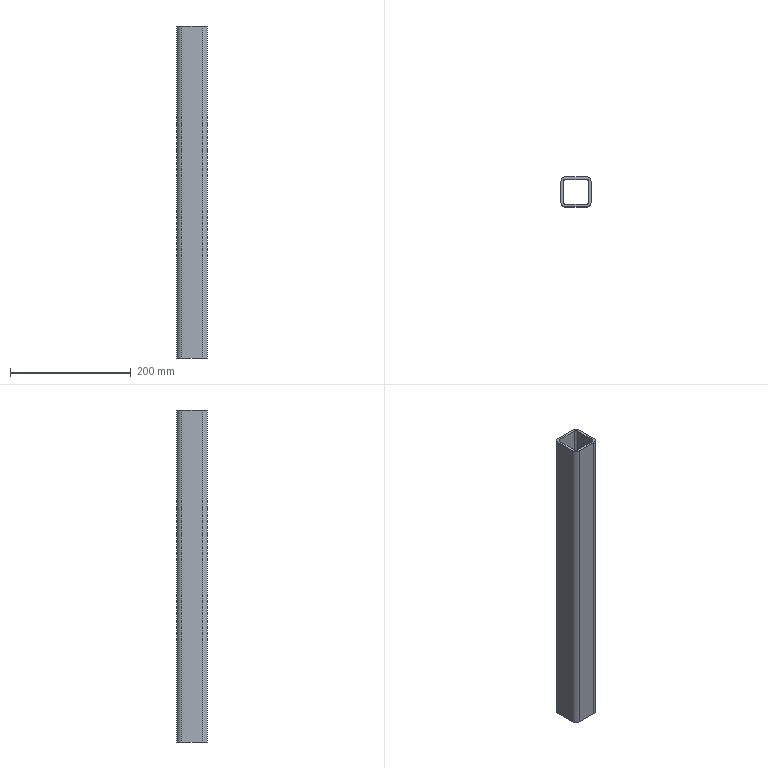Part | SolidWorks | features Extrusion 1 | 1 solid | 18 faces | box 50 x 50 x 550 mm | volume 382138 mm3 | plane 10 | cylinder 8 | commonest cylinder face diameters 8 x4 16 x4
STEP:
#1=CARTESIAN_POINT('',(17.,-25.,275.));
#2=VERTEX_POINT('',#1);
#3=CARTESIAN_POINT('',(25.,-17.,275.));
#4=VERTEX_POINT('',#3);
#5=CARTESIAN_POINT('',(17.,-17.,275.));
#6=DIRECTION('',(0.,0.,1.));
#7=DIRECTION('',(1.,0.,0.));
#8=AXIS2_PLACEMENT_3D('',#5,#6,#7);
#9=CIRCLE('',#8,8.);
#10=EDGE_CURVE('',#2,#4,#9,.T.);
#11=ORIENTED_EDGE('',*,*,#10,.T.);
#12=CARTESIAN_POINT('',(25.,17.,275.));
#13=VERTEX_POINT('',#12);
#14=CARTESIAN_POINT('',(25.,-17.,275.));
#15=DIRECTION('',(0.,1.,0.));
#16=VECTOR('',#15,1000.);
#17=LINE('',#14,#16);
#18=EDGE_CURVE('',#4,#13,#17,.T.);
#19=ORIENTED_EDGE('',*,*,#18,.T.);
#20=CARTESIAN_POINT('',(17.,25.,275.));
#21=VERTEX_POINT('',#20);
#22=CARTESIAN_POINT('',(17.,17.,275.));
#23=DIRECTION('',(0.,0.,1.));
#24=DIRECTION('',(-1.,0.,0.));
#25=AXIS2_PLACEMENT_3D('',#22,#23,#24);
#26=CIRCLE('',#25,8.);
#27=EDGE_CURVE('',#13,#21,#26,.T.);
#28=ORIENTED_EDGE('',*,*,#27,.T.);
#29=CARTESIAN_POINT('',(-17.,25.,275.));
#30=VERTEX_POINT('',#29);
#31=CARTESIAN_POINT('',(-17.,25.,275.));
#32=DIRECTION('',(-1.,0.,0.));
#33=VECTOR('',#32,1000.);
#34=LINE('',#31,#33);
#35=EDGE_CURVE('',#21,#30,#34,.T.);
#36=ORIENTED_EDGE('',*,*,#35,.T.);
#37=CARTESIAN_POINT('',(-25.,17.,275.));
#38=VERTEX_POINT('',#37);
#39=CARTESIAN_POINT('',(-17.,17.,275.));
#40=DIRECTION('',(0.,0.,1.));
#41=DIRECTION('',(-1.,0.,0.));
#42=AXIS2_PLACEMENT_3D('',#39,#40,#41);
#43=CIRCLE('',#42,8.);
#44=EDGE_CURVE('',#30,#38,#43,.T.);
#45=ORIENTED_EDGE('',*,*,#44,.T.);
#46=CARTESIAN_POINT('',(-25.,-17.,275.));
#47=VERTEX_POINT('',#46);
#48=CARTESIAN_POINT('',(-25.,-17.,275.));
#49=DIRECTION('',(0.,-1.,0.));
#50=VECTOR('',#49,1000.);
#51=LINE('',#48,#50);
#52=EDGE_CURVE('',#38,#47,#51,.T.);
#53=ORIENTED_EDGE('',*,*,#52,.T.);
#54=CARTESIAN_POINT('',(-17.,-25.,275.));
#55=VERTEX_POINT('',#54);
#56=CARTESIAN_POINT('',(-17.,-17.,275.));
#57=DIRECTION('',(0.,0.,1.));
#58=DIRECTION('',(-1.,0.,0.));
#59=AXIS2_PLACEMENT_3D('',#56,#57,#58);
#60=CIRCLE('',#59,8.);
#61=EDGE_CURVE('',#47,#55,#60,.T.);
#62=ORIENTED_EDGE('',*,*,#61,.T.);
#63=CARTESIAN_POINT('',(-17.,-25.,275.));
#64=DIRECTION('',(1.,0.,0.));
#65=VECTOR('',#64,1000.);
#66=LINE('',#63,#65);
#67=EDGE_CURVE('',#55,#2,#66,.T.);
#68=ORIENTED_EDGE('',*,*,#67,.T.);
#69=EDGE_LOOP('',(#11,#19,#28,#36,#45,#53,#62,#68));
#70=FACE_OUTER_BOUND('',#69,.T.);
#71=CARTESIAN_POINT('',(-21.,17.,275.));
#72=VERTEX_POINT('',#71);
#73=CARTESIAN_POINT('',(-21.,-17.,275.));
#74=VERTEX_POINT('',#73);
#75=CARTESIAN_POINT('',(-21.,-17.,275.));
#76=DIRECTION('',(0.,-1.,0.));
#77=VECTOR('',#76,1000.);
#78=LINE('',#75,#77);
#79=EDGE_CURVE('',#72,#74,#78,.T.);
#80=ORIENTED_EDGE('',*,*,#79,.F.);
#81=CARTESIAN_POINT('',(-17.,21.,275.));
#82=VERTEX_POINT('',#81);
#83=CARTESIAN_POINT('',(-17.,17.,275.));
#84=DIRECTION('',(0.,0.,1.));
#85=DIRECTION('',(-1.,0.,0.));
#86=AXIS2_PLACEMENT_3D('',#83,#84,#85);
#87=CIRCLE('',#86,4.);
#88=EDGE_CURVE('',#82,#72,#87,.T.);
#89=ORIENTED_EDGE('',*,*,#88,.F.);
#90=CARTESIAN_POINT('',(17.,21.,275.));
#91=VERTEX_POINT('',#90);
#92=CARTESIAN_POINT('',(-17.,21.,275.));
#93=DIRECTION('',(-1.,0.,0.));
#94=VECTOR('',#93,1000.);
#95=LINE('',#92,#94);
#96=EDGE_CURVE('',#91,#82,#95,.T.);
#97=ORIENTED_EDGE('',*,*,#96,.F.);
#98=CARTESIAN_POINT('',(21.,17.,275.));
#99=VERTEX_POINT('',#98);
#100=CARTESIAN_POINT('',(17.,17.,275.));
#101=DIRECTION('',(0.,0.,1.));
#102=DIRECTION('',(-1.,0.,0.));
#103=AXIS2_PLACEMENT_3D('',#100,#101,#102);
#104=CIRCLE('',#103,4.);
#105=EDGE_CURVE('',#99,#91,#104,.T.);
#106=ORIENTED_EDGE('',*,*,#105,.F.);
#107=CARTESIAN_POINT('',(21.,-17.,275.));
#108=VERTEX_POINT('',#107);
#109=CARTESIAN_POINT('',(21.,-17.,275.));
#110=DIRECTION('',(0.,1.,0.));
#111=VECTOR('',#110,1000.);
#112=LINE('',#109,#111);
#113=EDGE_CURVE('',#108,#99,#112,.T.);
#114=ORIENTED_EDGE('',*,*,#113,.F.);
#115=CARTESIAN_POINT('',(17.,-21.,275.));
#116=VERTEX_POINT('',#115);
#117=CARTESIAN_POINT('',(17.,-17.,275.));
#118=DIRECTION('',(0.,0.,1.));
#119=DIRECTION('',(1.,0.,0.));
#120=AXIS2_PLACEMENT_3D('',#117,#118,#119);
#121=CIRCLE('',#120,4.);
#122=EDGE_CURVE('',#116,#108,#121,.T.);
#123=ORIENTED_EDGE('',*,*,#122,.F.);
#124=CARTESIAN_POINT('',(-17.,-21.,275.));
#125=VERTEX_POINT('',#124);
#126=CARTESIAN_POINT('',(-17.,-21.,275.));
#127=DIRECTION('',(1.,0.,0.));
#128=VECTOR('',#127,1000.);
#129=LINE('',#126,#128);
#130=EDGE_CURVE('',#125,#116,#129,.T.);
#131=ORIENTED_EDGE('',*,*,#130,.F.);
#132=CARTESIAN_POINT('',(-17.,-17.,275.));
#133=DIRECTION('',(0.,0.,1.));
#134=DIRECTION('',(-1.,0.,0.));
#135=AXIS2_PLACEMENT_3D('',#132,#133,#134);
#136=CIRCLE('',#135,4.);
#137=EDGE_CURVE('',#74,#125,#136,.T.);
#138=ORIENTED_EDGE('',*,*,#137,.F.);
#139=EDGE_LOOP('',(#80,#89,#97,#106,#114,#123,#131,#138));
#140=FACE_BOUND('',#139,.T.);
#141=CARTESIAN_POINT('',(17.,-17.,275.));
#142=DIRECTION('',(0.,0.,1.));
#143=DIRECTION('',(1.,0.,0.));
#144=AXIS2_PLACEMENT_3D('',#141,#142,#143);
#145=PLANE('',#144);
#146=ADVANCED_FACE('',(#70,#140),#145,.T.);
#147=CARTESIAN_POINT('',(17.,-25.,-275.));
#148=VERTEX_POINT('',#147);
#149=CARTESIAN_POINT('',(25.,-17.,-275.));
#150=VERTEX_POINT('',#149);
#151=CARTESIAN_POINT('',(17.,-17.,-275.));
#152=DIRECTION('',(0.,0.,1.));
#153=DIRECTION('',(1.,0.,0.));
#154=AXIS2_PLACEMENT_3D('',#151,#152,#153);
#155=CIRCLE('',#154,8.);
#156=EDGE_CURVE('',#148,#150,#155,.T.);
#157=ORIENTED_EDGE('',*,*,#156,.F.);
#158=CARTESIAN_POINT('',(-17.,-25.,-275.));
#159=VERTEX_POINT('',#158);
#160=CARTESIAN_POINT('',(-17.,-25.,-275.));
#161=DIRECTION('',(1.,0.,0.));
#162=VECTOR('',#161,1000.);
#163=LINE('',#160,#162);
#164=EDGE_CURVE('',#159,#148,#163,.T.);
#165=ORIENTED_EDGE('',*,*,#164,.F.);
#166=CARTESIAN_POINT('',(-25.,-17.,-275.));
#167=VERTEX_POINT('',#166);
#168=CARTESIAN_POINT('',(-17.,-17.,-275.));
#169=DIRECTION('',(0.,0.,1.));
#170=DIRECTION('',(-1.,0.,0.));
#171=AXIS2_PLACEMENT_3D('',#168,#169,#170);
#172=CIRCLE('',#171,8.);
#173=EDGE_CURVE('',#167,#159,#172,.T.);
#174=ORIENTED_EDGE('',*,*,#173,.F.);
#175=CARTESIAN_POINT('',(-25.,17.,-275.));
#176=VERTEX_POINT('',#175);
#177=CARTESIAN_POINT('',(-25.,-17.,-275.));
#178=DIRECTION('',(0.,-1.,0.));
#179=VECTOR('',#178,1000.);
#180=LINE('',#177,#179);
#181=EDGE_CURVE('',#176,#167,#180,.T.);
#182=ORIENTED_EDGE('',*,*,#181,.F.);
#183=CARTESIAN_POINT('',(-17.,25.,-275.));
#184=VERTEX_POINT('',#183);
#185=CARTESIAN_POINT('',(-17.,17.,-275.));
#186=DIRECTION('',(0.,0.,1.));
#187=DIRECTION('',(-1.,0.,0.));
#188=AXIS2_PLACEMENT_3D('',#185,#186,#187);
#189=CIRCLE('',#188,8.);
#190=EDGE_CURVE('',#184,#176,#189,.T.);
#191=ORIENTED_EDGE('',*,*,#190,.F.);
#192=CARTESIAN_POINT('',(17.,25.,-275.));
#193=VERTEX_POINT('',#192);
#194=CARTESIAN_POINT('',(-17.,25.,-275.));
#195=DIRECTION('',(-1.,0.,0.));
#196=VECTOR('',#195,1000.);
#197=LINE('',#194,#196);
#198=EDGE_CURVE('',#193,#184,#197,.T.);
#199=ORIENTED_EDGE('',*,*,#198,.F.);
#200=CARTESIAN_POINT('',(25.,17.,-275.));
#201=VERTEX_POINT('',#200);
#202=CARTESIAN_POINT('',(17.,17.,-275.));
#203=DIRECTION('',(0.,0.,1.));
#204=DIRECTION('',(-1.,0.,0.));
#205=AXIS2_PLACEMENT_3D('',#202,#203,#204);
#206=CIRCLE('',#205,8.);
#207=EDGE_CURVE('',#201,#193,#206,.T.);
#208=ORIENTED_EDGE('',*,*,#207,.F.);
#209=CARTESIAN_POINT('',(25.,-17.,-275.));
#210=DIRECTION('',(0.,1.,0.));
#211=VECTOR('',#210,1000.);
#212=LINE('',#209,#211);
#213=EDGE_CURVE('',#150,#201,#212,.T.);
#214=ORIENTED_EDGE('',*,*,#213,.F.);
#215=EDGE_LOOP('',(#157,#165,#174,#182,#191,#199,#208,#214));
#216=FACE_OUTER_BOUND('',#215,.T.);
#217=CARTESIAN_POINT('',(-17.,21.,-275.));
#218=VERTEX_POINT('',#217);
#219=CARTESIAN_POINT('',(-21.,17.,-275.));
#220=VERTEX_POINT('',#219);
#221=CARTESIAN_POINT('',(-17.,17.,-275.));
#222=DIRECTION('',(0.,0.,1.));
#223=DIRECTION('',(-1.,0.,0.));
#224=AXIS2_PLACEMENT_3D('',#221,#222,#223);
#225=CIRCLE('',#224,4.);
#226=EDGE_CURVE('',#218,#220,#225,.T.);
#227=ORIENTED_EDGE('',*,*,#226,.T.);
#228=CARTESIAN_POINT('',(-21.,-17.,-275.));
#229=VERTEX_POINT('',#228);
#230=CARTESIAN_POINT('',(-21.,-17.,-275.));
#231=DIRECTION('',(0.,-1.,0.));
#232=VECTOR('',#231,1000.);
#233=LINE('',#230,#232);
#234=EDGE_CURVE('',#220,#229,#233,.T.);
#235=ORIENTED_EDGE('',*,*,#234,.T.);
#236=CARTESIAN_POINT('',(-17.,-21.,-275.));
#237=VERTEX_POINT('',#236);
#238=CARTESIAN_POINT('',(-17.,-17.,-275.));
#239=DIRECTION('',(0.,0.,1.));
#240=DIRECTION('',(-1.,0.,0.));
#241=AXIS2_PLACEMENT_3D('',#238,#239,#240);
#242=CIRCLE('',#241,4.);
#243=EDGE_CURVE('',#229,#237,#242,.T.);
#244=ORIENTED_EDGE('',*,*,#243,.T.);
#245=CARTESIAN_POINT('',(17.,-21.,-275.));
#246=VERTEX_POINT('',#245);
#247=CARTESIAN_POINT('',(-17.,-21.,-275.));
#248=DIRECTION('',(1.,0.,0.));
#249=VECTOR('',#248,1000.);
#250=LINE('',#247,#249);
#251=EDGE_CURVE('',#237,#246,#250,.T.);
#252=ORIENTED_EDGE('',*,*,#251,.T.);
#253=CARTESIAN_POINT('',(21.,-17.,-275.));
#254=VERTEX_POINT('',#253);
#255=CARTESIAN_POINT('',(17.,-17.,-275.));
#256=DIRECTION('',(0.,0.,1.));
#257=DIRECTION('',(1.,0.,0.));
#258=AXIS2_PLACEMENT_3D('',#255,#256,#257);
#259=CIRCLE('',#258,4.);
#260=EDGE_CURVE('',#246,#254,#259,.T.);
#261=ORIENTED_EDGE('',*,*,#260,.T.);
#262=CARTESIAN_POINT('',(21.,17.,-275.));
#263=VERTEX_POINT('',#262);
#264=CARTESIAN_POINT('',(21.,-17.,-275.));
#265=DIRECTION('',(0.,1.,0.));
#266=VECTOR('',#265,1000.);
#267=LINE('',#264,#266);
#268=EDGE_CURVE('',#254,#263,#267,.T.);
#269=ORIENTED_EDGE('',*,*,#268,.T.);
#270=CARTESIAN_POINT('',(17.,21.,-275.));
#271=VERTEX_POINT('',#270);
#272=CARTESIAN_POINT('',(17.,17.,-275.));
#273=DIRECTION('',(0.,0.,1.));
#274=DIRECTION('',(-1.,0.,0.));
#275=AXIS2_PLACEMENT_3D('',#272,#273,#274);
#276=CIRCLE('',#275,4.);
#277=EDGE_CURVE('',#263,#271,#276,.T.);
#278=ORIENTED_EDGE('',*,*,#277,.T.);
#279=CARTESIAN_POINT('',(-17.,21.,-275.));
#280=DIRECTION('',(-1.,0.,0.));
#281=VECTOR('',#280,1000.);
#282=LINE('',#279,#281);
#283=EDGE_CURVE('',#271,#218,#282,.T.);
#284=ORIENTED_EDGE('',*,*,#283,.T.);
#285=EDGE_LOOP('',(#227,#235,#244,#252,#261,#269,#278,#284));
#286=FACE_BOUND('',#285,.T.);
#287=CARTESIAN_POINT('',(17.,-17.,-275.));
#288=DIRECTION('',(0.,0.,1.));
#289=DIRECTION('',(1.,0.,0.));
#290=AXIS2_PLACEMENT_3D('',#287,#288,#289);
#291=PLANE('',#290);
#292=ADVANCED_FACE('',(#216,#286),#291,.F.);
#293=ORIENTED_EDGE('',*,*,#156,.T.);
#294=CARTESIAN_POINT('',(25.,-17.,275.));
#295=DIRECTION('',(0.,0.,-1.));
#296=VECTOR('',#295,1000.);
#297=LINE('',#294,#296);
#298=EDGE_CURVE('',#4,#150,#297,.T.);
#299=ORIENTED_EDGE('',*,*,#298,.F.);
#300=ORIENTED_EDGE('',*,*,#10,.F.);
#301=CARTESIAN_POINT('',(17.,-25.,275.));
#302=DIRECTION('',(0.,0.,-1.));
#303=VECTOR('',#302,1000.);
#304=LINE('',#301,#303);
#305=EDGE_CURVE('',#2,#148,#304,.T.);
#306=ORIENTED_EDGE('',*,*,#305,.T.);
#307=EDGE_LOOP('',(#293,#299,#300,#306));
#308=FACE_OUTER_BOUND('',#307,.T.);
#309=CARTESIAN_POINT('',(17.,-17.,275.));
#310=DIRECTION('',(0.,0.,-1.));
#311=DIRECTION('',(-1.,0.,0.));
#312=AXIS2_PLACEMENT_3D('',#309,#310,#311);
#313=CYLINDRICAL_SURFACE('',#312,8.);
#314=ADVANCED_FACE('',(#308),#313,.T.);
#315=ORIENTED_EDGE('',*,*,#213,.T.);
#316=CARTESIAN_POINT('',(25.,17.,275.));
#317=DIRECTION('',(0.,0.,-1.));
#318=VECTOR('',#317,1000.);
#319=LINE('',#316,#318);
#320=EDGE_CURVE('',#13,#201,#319,.T.);
#321=ORIENTED_EDGE('',*,*,#320,.F.);
#322=ORIENTED_EDGE('',*,*,#18,.F.);
#323=ORIENTED_EDGE('',*,*,#298,.T.);
#324=EDGE_LOOP('',(#315,#321,#322,#323));
#325=FACE_OUTER_BOUND('',#324,.T.);
#326=CARTESIAN_POINT('',(25.,-17.,275.));
#327=DIRECTION('',(-1.,0.,0.));
#328=DIRECTION('',(0.,0.,1.));
#329=AXIS2_PLACEMENT_3D('',#326,#327,#328);
#330=PLANE('',#329);
#331=ADVANCED_FACE('',(#325),#330,.F.);
#332=ORIENTED_EDGE('',*,*,#207,.T.);
#333=CARTESIAN_POINT('',(17.,25.,275.));
#334=DIRECTION('',(0.,0.,-1.));
#335=VECTOR('',#334,1000.);
#336=LINE('',#333,#335);
#337=EDGE_CURVE('',#21,#193,#336,.T.);
#338=ORIENTED_EDGE('',*,*,#337,.F.);
#339=ORIENTED_EDGE('',*,*,#27,.F.);
#340=ORIENTED_EDGE('',*,*,#320,.T.);
#341=EDGE_LOOP('',(#332,#338,#339,#340));
#342=FACE_OUTER_BOUND('',#341,.T.);
#343=CARTESIAN_POINT('',(17.,17.,275.));
#344=DIRECTION('',(0.,0.,-1.));
#345=DIRECTION('',(-1.,0.,0.));
#346=AXIS2_PLACEMENT_3D('',#343,#344,#345);
#347=CYLINDRICAL_SURFACE('',#346,8.);
#348=ADVANCED_FACE('',(#342),#347,.T.);
#349=ORIENTED_EDGE('',*,*,#198,.T.);
#350=CARTESIAN_POINT('',(-17.,25.,275.));
#351=DIRECTION('',(0.,0.,-1.));
#352=VECTOR('',#351,1000.);
#353=LINE('',#350,#352);
#354=EDGE_CURVE('',#30,#184,#353,.T.);
#355=ORIENTED_EDGE('',*,*,#354,.F.);
#356=ORIENTED_EDGE('',*,*,#35,.F.);
#357=ORIENTED_EDGE('',*,*,#337,.T.);
#358=EDGE_LOOP('',(#349,#355,#356,#357));
#359=FACE_OUTER_BOUND('',#358,.T.);
#360=CARTESIAN_POINT('',(-17.,25.,275.));
#361=DIRECTION('',(0.,-1.,0.));
#362=DIRECTION('',(0.,0.,-1.));
#363=AXIS2_PLACEMENT_3D('',#360,#361,#362);
#364=PLANE('',#363);
#365=ADVANCED_FACE('',(#359),#364,.F.);
#366=ORIENTED_EDGE('',*,*,#190,.T.);
#367=CARTESIAN_POINT('',(-25.,17.,275.));
#368=DIRECTION('',(0.,0.,-1.));
#369=VECTOR('',#368,1000.);
#370=LINE('',#367,#369);
#371=EDGE_CURVE('',#38,#176,#370,.T.);
#372=ORIENTED_EDGE('',*,*,#371,.F.);
#373=ORIENTED_EDGE('',*,*,#44,.F.);
#374=ORIENTED_EDGE('',*,*,#354,.T.);
#375=EDGE_LOOP('',(#366,#372,#373,#374));
#376=FACE_OUTER_BOUND('',#375,.T.);
#377=CARTESIAN_POINT('',(-17.,17.,275.));
#378=DIRECTION('',(0.,0.,-1.));
#379=DIRECTION('',(-1.,0.,0.));
#380=AXIS2_PLACEMENT_3D('',#377,#378,#379);
#381=CYLINDRICAL_SURFACE('',#380,8.);
#382=ADVANCED_FACE('',(#376),#381,.T.);
#383=ORIENTED_EDGE('',*,*,#181,.T.);
#384=CARTESIAN_POINT('',(-25.,-17.,275.));
#385=DIRECTION('',(0.,0.,-1.));
#386=VECTOR('',#385,1000.);
#387=LINE('',#384,#386);
#388=EDGE_CURVE('',#47,#167,#387,.T.);
#389=ORIENTED_EDGE('',*,*,#388,.F.);
#390=ORIENTED_EDGE('',*,*,#52,.F.);
#391=ORIENTED_EDGE('',*,*,#371,.T.);
#392=EDGE_LOOP('',(#383,#389,#390,#391));
#393=FACE_OUTER_BOUND('',#392,.T.);
#394=CARTESIAN_POINT('',(-25.,-17.,275.));
#395=DIRECTION('',(1.,0.,0.));
#396=DIRECTION('',(0.,0.,-1.));
#397=AXIS2_PLACEMENT_3D('',#394,#395,#396);
#398=PLANE('',#397);
#399=ADVANCED_FACE('',(#393),#398,.F.);
#400=ORIENTED_EDGE('',*,*,#173,.T.);
#401=CARTESIAN_POINT('',(-17.,-25.,275.));
#402=DIRECTION('',(0.,0.,-1.));
#403=VECTOR('',#402,1000.);
#404=LINE('',#401,#403);
#405=EDGE_CURVE('',#55,#159,#404,.T.);
#406=ORIENTED_EDGE('',*,*,#405,.F.);
#407=ORIENTED_EDGE('',*,*,#61,.F.);
#408=ORIENTED_EDGE('',*,*,#388,.T.);
#409=EDGE_LOOP('',(#400,#406,#407,#408));
#410=FACE_OUTER_BOUND('',#409,.T.);
#411=CARTESIAN_POINT('',(-17.,-17.,275.));
#412=DIRECTION('',(0.,0.,-1.));
#413=DIRECTION('',(-1.,0.,0.));
#414=AXIS2_PLACEMENT_3D('',#411,#412,#413);
#415=CYLINDRICAL_SURFACE('',#414,8.);
#416=ADVANCED_FACE('',(#410),#415,.T.);
#417=ORIENTED_EDGE('',*,*,#164,.T.);
#418=ORIENTED_EDGE('',*,*,#305,.F.);
#419=ORIENTED_EDGE('',*,*,#67,.F.);
#420=ORIENTED_EDGE('',*,*,#405,.T.);
#421=EDGE_LOOP('',(#417,#418,#419,#420));
#422=FACE_OUTER_BOUND('',#421,.T.);
#423=CARTESIAN_POINT('',(-17.,-25.,275.));
#424=DIRECTION('',(0.,1.,0.));
#425=DIRECTION('',(0.,0.,1.));
#426=AXIS2_PLACEMENT_3D('',#423,#424,#425);
#427=PLANE('',#426);
#428=ADVANCED_FACE('',(#422),#427,.F.);
#429=ORIENTED_EDGE('',*,*,#226,.F.);
#430=CARTESIAN_POINT('',(-17.,21.,275.));
#431=DIRECTION('',(0.,0.,-1.));
#432=VECTOR('',#431,1000.);
#433=LINE('',#430,#432);
#434=EDGE_CURVE('',#82,#218,#433,.T.);
#435=ORIENTED_EDGE('',*,*,#434,.F.);
#436=ORIENTED_EDGE('',*,*,#88,.T.);
#437=CARTESIAN_POINT('',(-21.,17.,275.));
#438=DIRECTION('',(0.,0.,-1.));
#439=VECTOR('',#438,1000.);
#440=LINE('',#437,#439);
#441=EDGE_CURVE('',#72,#220,#440,.T.);
#442=ORIENTED_EDGE('',*,*,#441,.T.);
#443=EDGE_LOOP('',(#429,#435,#436,#442));
#444=FACE_OUTER_BOUND('',#443,.T.);
#445=CARTESIAN_POINT('',(-17.,17.,275.));
#446=DIRECTION('',(0.,0.,-1.));
#447=DIRECTION('',(-1.,0.,0.));
#448=AXIS2_PLACEMENT_3D('',#445,#446,#447);
#449=CYLINDRICAL_SURFACE('',#448,4.);
#450=ADVANCED_FACE('',(#444),#449,.F.);
#451=ORIENTED_EDGE('',*,*,#234,.F.);
#452=ORIENTED_EDGE('',*,*,#441,.F.);
#453=ORIENTED_EDGE('',*,*,#79,.T.);
#454=CARTESIAN_POINT('',(-21.,-17.,275.));
#455=DIRECTION('',(0.,0.,-1.));
#456=VECTOR('',#455,1000.);
#457=LINE('',#454,#456);
#458=EDGE_CURVE('',#74,#229,#457,.T.);
#459=ORIENTED_EDGE('',*,*,#458,.T.);
#460=EDGE_LOOP('',(#451,#452,#453,#459));
#461=FACE_OUTER_BOUND('',#460,.T.);
#462=CARTESIAN_POINT('',(-21.,-17.,275.));
#463=DIRECTION('',(1.,0.,0.));
#464=DIRECTION('',(0.,0.,-1.));
#465=AXIS2_PLACEMENT_3D('',#462,#463,#464);
#466=PLANE('',#465);
#467=ADVANCED_FACE('',(#461),#466,.T.);
#468=ORIENTED_EDGE('',*,*,#243,.F.);
#469=ORIENTED_EDGE('',*,*,#458,.F.);
#470=ORIENTED_EDGE('',*,*,#137,.T.);
#471=CARTESIAN_POINT('',(-17.,-21.,275.));
#472=DIRECTION('',(0.,0.,-1.));
#473=VECTOR('',#472,1000.);
#474=LINE('',#471,#473);
#475=EDGE_CURVE('',#125,#237,#474,.T.);
#476=ORIENTED_EDGE('',*,*,#475,.T.);
#477=EDGE_LOOP('',(#468,#469,#470,#476));
#478=FACE_OUTER_BOUND('',#477,.T.);
#479=CARTESIAN_POINT('',(-17.,-17.,275.));
#480=DIRECTION('',(0.,0.,-1.));
#481=DIRECTION('',(-1.,0.,0.));
#482=AXIS2_PLACEMENT_3D('',#479,#480,#481);
#483=CYLINDRICAL_SURFACE('',#482,4.);
#484=ADVANCED_FACE('',(#478),#483,.F.);
#485=ORIENTED_EDGE('',*,*,#251,.F.);
#486=ORIENTED_EDGE('',*,*,#475,.F.);
#487=ORIENTED_EDGE('',*,*,#130,.T.);
#488=CARTESIAN_POINT('',(17.,-21.,275.));
#489=DIRECTION('',(0.,0.,-1.));
#490=VECTOR('',#489,1000.);
#491=LINE('',#488,#490);
#492=EDGE_CURVE('',#116,#246,#491,.T.);
#493=ORIENTED_EDGE('',*,*,#492,.T.);
#494=EDGE_LOOP('',(#485,#486,#487,#493));
#495=FACE_OUTER_BOUND('',#494,.T.);
#496=CARTESIAN_POINT('',(-17.,-21.,275.));
#497=DIRECTION('',(0.,1.,0.));
#498=DIRECTION('',(0.,0.,1.));
#499=AXIS2_PLACEMENT_3D('',#496,#497,#498);
#500=PLANE('',#499);
#501=ADVANCED_FACE('',(#495),#500,.T.);
#502=ORIENTED_EDGE('',*,*,#260,.F.);
#503=ORIENTED_EDGE('',*,*,#492,.F.);
#504=ORIENTED_EDGE('',*,*,#122,.T.);
#505=CARTESIAN_POINT('',(21.,-17.,275.));
#506=DIRECTION('',(0.,0.,-1.));
#507=VECTOR('',#506,1000.);
#508=LINE('',#505,#507);
#509=EDGE_CURVE('',#108,#254,#508,.T.);
#510=ORIENTED_EDGE('',*,*,#509,.T.);
#511=EDGE_LOOP('',(#502,#503,#504,#510));
#512=FACE_OUTER_BOUND('',#511,.T.);
#513=CARTESIAN_POINT('',(17.,-17.,275.));
#514=DIRECTION('',(0.,0.,-1.));
#515=DIRECTION('',(-1.,0.,0.));
#516=AXIS2_PLACEMENT_3D('',#513,#514,#515);
#517=CYLINDRICAL_SURFACE('',#516,4.);
#518=ADVANCED_FACE('',(#512),#517,.F.);
#519=ORIENTED_EDGE('',*,*,#268,.F.);
#520=ORIENTED_EDGE('',*,*,#509,.F.);
#521=ORIENTED_EDGE('',*,*,#113,.T.);
#522=CARTESIAN_POINT('',(21.,17.,275.));
#523=DIRECTION('',(0.,0.,-1.));
#524=VECTOR('',#523,1000.);
#525=LINE('',#522,#524);
#526=EDGE_CURVE('',#99,#263,#525,.T.);
#527=ORIENTED_EDGE('',*,*,#526,.T.);
#528=EDGE_LOOP('',(#519,#520,#521,#527));
#529=FACE_OUTER_BOUND('',#528,.T.);
#530=CARTESIAN_POINT('',(21.,-17.,275.));
#531=DIRECTION('',(-1.,0.,0.));
#532=DIRECTION('',(0.,0.,1.));
#533=AXIS2_PLACEMENT_3D('',#530,#531,#532);
#534=PLANE('',#533);
#535=ADVANCED_FACE('',(#529),#534,.T.);
#536=ORIENTED_EDGE('',*,*,#277,.F.);
#537=ORIENTED_EDGE('',*,*,#526,.F.);
#538=ORIENTED_EDGE('',*,*,#105,.T.);
#539=CARTESIAN_POINT('',(17.,21.,275.));
#540=DIRECTION('',(0.,0.,-1.));
#541=VECTOR('',#540,1000.);
#542=LINE('',#539,#541);
#543=EDGE_CURVE('',#91,#271,#542,.T.);
#544=ORIENTED_EDGE('',*,*,#543,.T.);
#545=EDGE_LOOP('',(#536,#537,#538,#544));
#546=FACE_OUTER_BOUND('',#545,.T.);
#547=CARTESIAN_POINT('',(17.,17.,275.));
#548=DIRECTION('',(0.,0.,-1.));
#549=DIRECTION('',(-1.,0.,0.));
#550=AXIS2_PLACEMENT_3D('',#547,#548,#549);
#551=CYLINDRICAL_SURFACE('',#550,4.);
#552=ADVANCED_FACE('',(#546),#551,.F.);
#553=ORIENTED_EDGE('',*,*,#283,.F.);
#554=ORIENTED_EDGE('',*,*,#543,.F.);
#555=ORIENTED_EDGE('',*,*,#96,.T.);
#556=ORIENTED_EDGE('',*,*,#434,.T.);
#557=EDGE_LOOP('',(#553,#554,#555,#556));
#558=FACE_OUTER_BOUND('',#557,.T.);
#559=CARTESIAN_POINT('',(-17.,21.,275.));
#560=DIRECTION('',(0.,-1.,0.));
#561=DIRECTION('',(0.,0.,-1.));
#562=AXIS2_PLACEMENT_3D('',#559,#560,#561);
#563=PLANE('',#562);
#564=ADVANCED_FACE('',(#558),#563,.T.);
#565=CLOSED_SHELL('',(#146,#292,#314,#331,#348,#365,#382,#399,#416,#428,#450,#467,#484,#501,#518,#535,#552,#564));
#566=MANIFOLD_SOLID_BREP('',#565);
#567=CARTESIAN_POINT('',(0.,0.,0.));
#568=DIRECTION('',(0.,0.,1.));
#569=DIRECTION('',(1.,0.,0.));
#570=AXIS2_PLACEMENT_3D('',#567,#568,#569);
#571=(LENGTH_UNIT()NAMED_UNIT(*)SI_UNIT(.MILLI.,.METRE.));
#572=UNCERTAINTY_MEASURE_WITH_UNIT(LENGTH_MEASURE(0.00001),#571,'','');
#573=(NAMED_UNIT(*)PLANE_ANGLE_UNIT()SI_UNIT($,.RADIAN.));
#574=(NAMED_UNIT(*)SI_UNIT($,.STERADIAN.)SOLID_ANGLE_UNIT());
#575=(GEOMETRIC_REPRESENTATION_CONTEXT(3)GLOBAL_UNCERTAINTY_ASSIGNED_CONTEXT((#572))GLOBAL_UNIT_ASSIGNED_CONTEXT((#571,#573,#574))REPRESENTATION_CONTEXT('',''));
#576=ADVANCED_BREP_SHAPE_REPRESENTATION('',(#566,#570),#575);